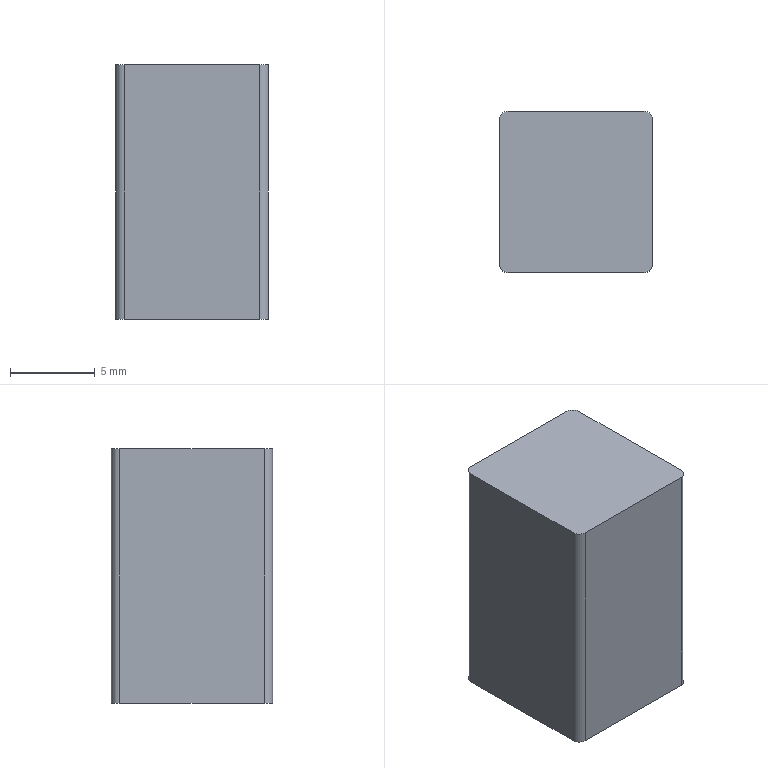Part | NX | features BREP 1 | 1 solid | 10 faces | box 9.003 x 9.506 x 15 mm | volume 1281 mm3 | plane 6 | cylinder 4 | commonest cylinder face diameters 1 x4
STEP:
#1=CARTESIAN_POINT('',(-4.002,4.753,-25.6));
#2=VERTEX_POINT('',#1);
#3=CARTESIAN_POINT('',(-4.502,4.253,-25.6));
#4=VERTEX_POINT('',#3);
#5=CARTESIAN_POINT('',(-4.002,4.253,-25.6));
#6=DIRECTION('',(0.,0.,1.));
#7=DIRECTION('',(1.,0.,0.));
#8=AXIS2_PLACEMENT_3D('',#5,#6,#7);
#9=CIRCLE('',#8,0.5);
#10=EDGE_CURVE('',#2,#4,#9,.T.);
#11=ORIENTED_EDGE('',*,*,#10,.F.);
#12=CARTESIAN_POINT('',(-4.002,4.753,-40.6));
#13=VERTEX_POINT('',#12);
#14=CARTESIAN_POINT('',(-4.002,4.753,-40.6));
#15=DIRECTION('',(0.,0.,1.));
#16=VECTOR('',#15,1000.);
#17=LINE('',#14,#16);
#18=EDGE_CURVE('',#13,#2,#17,.T.);
#19=ORIENTED_EDGE('',*,*,#18,.F.);
#20=CARTESIAN_POINT('',(-4.502,4.253,-40.6));
#21=VERTEX_POINT('',#20);
#22=CARTESIAN_POINT('',(-4.002,4.253,-40.6));
#23=DIRECTION('',(0.,0.,1.));
#24=DIRECTION('',(1.,0.,0.));
#25=AXIS2_PLACEMENT_3D('',#22,#23,#24);
#26=CIRCLE('',#25,0.5);
#27=EDGE_CURVE('',#13,#21,#26,.T.);
#28=ORIENTED_EDGE('',*,*,#27,.T.);
#29=CARTESIAN_POINT('',(-4.502,4.253,-40.6));
#30=DIRECTION('',(0.,0.,1.));
#31=VECTOR('',#30,1000.);
#32=LINE('',#29,#31);
#33=EDGE_CURVE('',#21,#4,#32,.T.);
#34=ORIENTED_EDGE('',*,*,#33,.T.);
#35=EDGE_LOOP('',(#11,#19,#28,#34));
#36=FACE_BOUND('',#35,.T.);
#37=CARTESIAN_POINT('',(-4.002,4.253,-40.6));
#38=DIRECTION('',(0.,0.,1.));
#39=DIRECTION('',(-1.,0.,0.));
#40=AXIS2_PLACEMENT_3D('',#37,#38,#39);
#41=CYLINDRICAL_SURFACE('',#40,0.5);
#42=ADVANCED_FACE('',(#36),#41,.T.);
#43=CARTESIAN_POINT('',(-4.502,-4.253,-25.6));
#44=VERTEX_POINT('',#43);
#45=CARTESIAN_POINT('',(-4.502,-4.253,-25.6));
#46=DIRECTION('',(0.,1.,0.));
#47=VECTOR('',#46,1000.);
#48=LINE('',#45,#47);
#49=EDGE_CURVE('',#44,#4,#48,.T.);
#50=ORIENTED_EDGE('',*,*,#49,.T.);
#51=ORIENTED_EDGE('',*,*,#33,.F.);
#52=CARTESIAN_POINT('',(-4.502,-4.253,-40.6));
#53=VERTEX_POINT('',#52);
#54=CARTESIAN_POINT('',(-4.502,-4.253,-40.6));
#55=DIRECTION('',(0.,1.,0.));
#56=VECTOR('',#55,1000.);
#57=LINE('',#54,#56);
#58=EDGE_CURVE('',#53,#21,#57,.T.);
#59=ORIENTED_EDGE('',*,*,#58,.F.);
#60=CARTESIAN_POINT('',(-4.502,-4.253,-40.6));
#61=DIRECTION('',(0.,0.,1.));
#62=VECTOR('',#61,1000.);
#63=LINE('',#60,#62);
#64=EDGE_CURVE('',#53,#44,#63,.T.);
#65=ORIENTED_EDGE('',*,*,#64,.T.);
#66=EDGE_LOOP('',(#50,#51,#59,#65));
#67=FACE_BOUND('',#66,.T.);
#68=CARTESIAN_POINT('',(-4.502,-4.253,-40.6));
#69=DIRECTION('',(1.,0.,0.));
#70=DIRECTION('',(0.,-1.,0.));
#71=AXIS2_PLACEMENT_3D('',#68,#69,#70);
#72=PLANE('',#71);
#73=ADVANCED_FACE('',(#67),#72,.F.);
#74=CARTESIAN_POINT('',(-4.002,-4.753,-25.6));
#75=VERTEX_POINT('',#74);
#76=CARTESIAN_POINT('',(-4.002,-4.253,-25.6));
#77=DIRECTION('',(0.,0.,1.));
#78=DIRECTION('',(1.,0.,0.));
#79=AXIS2_PLACEMENT_3D('',#76,#77,#78);
#80=CIRCLE('',#79,0.5);
#81=EDGE_CURVE('',#44,#75,#80,.T.);
#82=ORIENTED_EDGE('',*,*,#81,.F.);
#83=ORIENTED_EDGE('',*,*,#64,.F.);
#84=CARTESIAN_POINT('',(-4.002,-4.753,-40.6));
#85=VERTEX_POINT('',#84);
#86=CARTESIAN_POINT('',(-4.002,-4.253,-40.6));
#87=DIRECTION('',(0.,0.,1.));
#88=DIRECTION('',(1.,0.,0.));
#89=AXIS2_PLACEMENT_3D('',#86,#87,#88);
#90=CIRCLE('',#89,0.5);
#91=EDGE_CURVE('',#53,#85,#90,.T.);
#92=ORIENTED_EDGE('',*,*,#91,.T.);
#93=CARTESIAN_POINT('',(-4.002,-4.753,-40.6));
#94=DIRECTION('',(0.,0.,1.));
#95=VECTOR('',#94,1000.);
#96=LINE('',#93,#95);
#97=EDGE_CURVE('',#85,#75,#96,.T.);
#98=ORIENTED_EDGE('',*,*,#97,.T.);
#99=EDGE_LOOP('',(#82,#83,#92,#98));
#100=FACE_BOUND('',#99,.T.);
#101=CARTESIAN_POINT('',(-4.002,-4.253,-40.6));
#102=DIRECTION('',(0.,0.,1.));
#103=DIRECTION('',(-1.,0.,0.));
#104=AXIS2_PLACEMENT_3D('',#101,#102,#103);
#105=CYLINDRICAL_SURFACE('',#104,0.5);
#106=ADVANCED_FACE('',(#100),#105,.T.);
#107=CARTESIAN_POINT('',(4.002,-4.753,-25.6));
#108=VERTEX_POINT('',#107);
#109=CARTESIAN_POINT('',(4.002,-4.753,-25.6));
#110=DIRECTION('',(-1.,0.,0.));
#111=VECTOR('',#110,1000.);
#112=LINE('',#109,#111);
#113=EDGE_CURVE('',#108,#75,#112,.T.);
#114=ORIENTED_EDGE('',*,*,#113,.T.);
#115=ORIENTED_EDGE('',*,*,#97,.F.);
#116=CARTESIAN_POINT('',(4.002,-4.753,-40.6));
#117=VERTEX_POINT('',#116);
#118=CARTESIAN_POINT('',(4.002,-4.753,-40.6));
#119=DIRECTION('',(-1.,0.,0.));
#120=VECTOR('',#119,1000.);
#121=LINE('',#118,#120);
#122=EDGE_CURVE('',#117,#85,#121,.T.);
#123=ORIENTED_EDGE('',*,*,#122,.F.);
#124=CARTESIAN_POINT('',(4.002,-4.753,-40.6));
#125=DIRECTION('',(0.,0.,1.));
#126=VECTOR('',#125,1000.);
#127=LINE('',#124,#126);
#128=EDGE_CURVE('',#117,#108,#127,.T.);
#129=ORIENTED_EDGE('',*,*,#128,.T.);
#130=EDGE_LOOP('',(#114,#115,#123,#129));
#131=FACE_BOUND('',#130,.T.);
#132=CARTESIAN_POINT('',(4.002,-4.753,-40.6));
#133=DIRECTION('',(0.,1.,0.));
#134=DIRECTION('',(1.,0.,0.));
#135=AXIS2_PLACEMENT_3D('',#132,#133,#134);
#136=PLANE('',#135);
#137=ADVANCED_FACE('',(#131),#136,.F.);
#138=CARTESIAN_POINT('',(4.502,-4.253,-25.6));
#139=VERTEX_POINT('',#138);
#140=CARTESIAN_POINT('',(4.002,-4.253,-25.6));
#141=DIRECTION('',(0.,0.,1.));
#142=DIRECTION('',(1.,0.,0.));
#143=AXIS2_PLACEMENT_3D('',#140,#141,#142);
#144=CIRCLE('',#143,0.5);
#145=EDGE_CURVE('',#108,#139,#144,.T.);
#146=ORIENTED_EDGE('',*,*,#145,.F.);
#147=ORIENTED_EDGE('',*,*,#128,.F.);
#148=CARTESIAN_POINT('',(4.502,-4.253,-40.6));
#149=VERTEX_POINT('',#148);
#150=CARTESIAN_POINT('',(4.002,-4.253,-40.6));
#151=DIRECTION('',(0.,0.,1.));
#152=DIRECTION('',(1.,0.,0.));
#153=AXIS2_PLACEMENT_3D('',#150,#151,#152);
#154=CIRCLE('',#153,0.5);
#155=EDGE_CURVE('',#117,#149,#154,.T.);
#156=ORIENTED_EDGE('',*,*,#155,.T.);
#157=CARTESIAN_POINT('',(4.502,-4.253,-40.6));
#158=DIRECTION('',(0.,0.,1.));
#159=VECTOR('',#158,1000.);
#160=LINE('',#157,#159);
#161=EDGE_CURVE('',#149,#139,#160,.T.);
#162=ORIENTED_EDGE('',*,*,#161,.T.);
#163=EDGE_LOOP('',(#146,#147,#156,#162));
#164=FACE_BOUND('',#163,.T.);
#165=CARTESIAN_POINT('',(4.002,-4.253,-40.6));
#166=DIRECTION('',(0.,0.,1.));
#167=DIRECTION('',(-1.,0.,0.));
#168=AXIS2_PLACEMENT_3D('',#165,#166,#167);
#169=CYLINDRICAL_SURFACE('',#168,0.5);
#170=ADVANCED_FACE('',(#164),#169,.T.);
#171=CARTESIAN_POINT('',(4.502,4.253,-25.6));
#172=VERTEX_POINT('',#171);
#173=CARTESIAN_POINT('',(4.502,4.253,-25.6));
#174=DIRECTION('',(0.,-1.,0.));
#175=VECTOR('',#174,1000.);
#176=LINE('',#173,#175);
#177=EDGE_CURVE('',#172,#139,#176,.T.);
#178=ORIENTED_EDGE('',*,*,#177,.T.);
#179=ORIENTED_EDGE('',*,*,#161,.F.);
#180=CARTESIAN_POINT('',(4.502,4.253,-40.6));
#181=VERTEX_POINT('',#180);
#182=CARTESIAN_POINT('',(4.502,4.253,-40.6));
#183=DIRECTION('',(0.,-1.,0.));
#184=VECTOR('',#183,1000.);
#185=LINE('',#182,#184);
#186=EDGE_CURVE('',#181,#149,#185,.T.);
#187=ORIENTED_EDGE('',*,*,#186,.F.);
#188=CARTESIAN_POINT('',(4.502,4.253,-40.6));
#189=DIRECTION('',(0.,0.,1.));
#190=VECTOR('',#189,1000.);
#191=LINE('',#188,#190);
#192=EDGE_CURVE('',#181,#172,#191,.T.);
#193=ORIENTED_EDGE('',*,*,#192,.T.);
#194=EDGE_LOOP('',(#178,#179,#187,#193));
#195=FACE_BOUND('',#194,.T.);
#196=CARTESIAN_POINT('',(4.502,4.253,-40.6));
#197=DIRECTION('',(-1.,0.,0.));
#198=DIRECTION('',(0.,1.,0.));
#199=AXIS2_PLACEMENT_3D('',#196,#197,#198);
#200=PLANE('',#199);
#201=ADVANCED_FACE('',(#195),#200,.F.);
#202=CARTESIAN_POINT('',(4.002,4.753,-25.6));
#203=VERTEX_POINT('',#202);
#204=CARTESIAN_POINT('',(4.002,4.253,-25.6));
#205=DIRECTION('',(0.,0.,1.));
#206=DIRECTION('',(1.,0.,0.));
#207=AXIS2_PLACEMENT_3D('',#204,#205,#206);
#208=CIRCLE('',#207,0.5);
#209=EDGE_CURVE('',#172,#203,#208,.T.);
#210=ORIENTED_EDGE('',*,*,#209,.F.);
#211=ORIENTED_EDGE('',*,*,#192,.F.);
#212=CARTESIAN_POINT('',(4.002,4.753,-40.6));
#213=VERTEX_POINT('',#212);
#214=CARTESIAN_POINT('',(4.002,4.253,-40.6));
#215=DIRECTION('',(0.,0.,1.));
#216=DIRECTION('',(1.,0.,0.));
#217=AXIS2_PLACEMENT_3D('',#214,#215,#216);
#218=CIRCLE('',#217,0.5);
#219=EDGE_CURVE('',#181,#213,#218,.T.);
#220=ORIENTED_EDGE('',*,*,#219,.T.);
#221=CARTESIAN_POINT('',(4.002,4.753,-40.6));
#222=DIRECTION('',(0.,0.,1.));
#223=VECTOR('',#222,1000.);
#224=LINE('',#221,#223);
#225=EDGE_CURVE('',#213,#203,#224,.T.);
#226=ORIENTED_EDGE('',*,*,#225,.T.);
#227=EDGE_LOOP('',(#210,#211,#220,#226));
#228=FACE_BOUND('',#227,.T.);
#229=CARTESIAN_POINT('',(4.002,4.253,-40.6));
#230=DIRECTION('',(0.,0.,1.));
#231=DIRECTION('',(-1.,0.,0.));
#232=AXIS2_PLACEMENT_3D('',#229,#230,#231);
#233=CYLINDRICAL_SURFACE('',#232,0.5);
#234=ADVANCED_FACE('',(#228),#233,.T.);
#235=CARTESIAN_POINT('',(-4.002,4.753,-25.6));
#236=DIRECTION('',(1.,0.,0.));
#237=VECTOR('',#236,1000.);
#238=LINE('',#235,#237);
#239=EDGE_CURVE('',#2,#203,#238,.T.);
#240=ORIENTED_EDGE('',*,*,#239,.T.);
#241=ORIENTED_EDGE('',*,*,#225,.F.);
#242=CARTESIAN_POINT('',(-4.002,4.753,-40.6));
#243=DIRECTION('',(1.,0.,0.));
#244=VECTOR('',#243,1000.);
#245=LINE('',#242,#244);
#246=EDGE_CURVE('',#13,#213,#245,.T.);
#247=ORIENTED_EDGE('',*,*,#246,.F.);
#248=ORIENTED_EDGE('',*,*,#18,.T.);
#249=EDGE_LOOP('',(#240,#241,#247,#248));
#250=FACE_BOUND('',#249,.T.);
#251=CARTESIAN_POINT('',(-4.002,4.753,-40.6));
#252=DIRECTION('',(0.,-1.,0.));
#253=DIRECTION('',(0.,0.,1.));
#254=AXIS2_PLACEMENT_3D('',#251,#252,#253);
#255=PLANE('',#254);
#256=ADVANCED_FACE('',(#250),#255,.F.);
#257=ORIENTED_EDGE('',*,*,#27,.F.);
#258=ORIENTED_EDGE('',*,*,#246,.T.);
#259=ORIENTED_EDGE('',*,*,#219,.F.);
#260=ORIENTED_EDGE('',*,*,#186,.T.);
#261=ORIENTED_EDGE('',*,*,#155,.F.);
#262=ORIENTED_EDGE('',*,*,#122,.T.);
#263=ORIENTED_EDGE('',*,*,#91,.F.);
#264=ORIENTED_EDGE('',*,*,#58,.T.);
#265=EDGE_LOOP('',(#257,#258,#259,#260,#261,#262,#263,#264));
#266=FACE_BOUND('',#265,.T.);
#267=CARTESIAN_POINT('',(-4.002,4.253,-40.6));
#268=DIRECTION('',(0.,0.,1.));
#269=DIRECTION('',(-1.,0.,0.));
#270=AXIS2_PLACEMENT_3D('',#267,#268,#269);
#271=PLANE('',#270);
#272=ADVANCED_FACE('',(#266),#271,.F.);
#273=ORIENTED_EDGE('',*,*,#10,.T.);
#274=ORIENTED_EDGE('',*,*,#49,.F.);
#275=ORIENTED_EDGE('',*,*,#81,.T.);
#276=ORIENTED_EDGE('',*,*,#113,.F.);
#277=ORIENTED_EDGE('',*,*,#145,.T.);
#278=ORIENTED_EDGE('',*,*,#177,.F.);
#279=ORIENTED_EDGE('',*,*,#209,.T.);
#280=ORIENTED_EDGE('',*,*,#239,.F.);
#281=EDGE_LOOP('',(#273,#274,#275,#276,#277,#278,#279,#280));
#282=FACE_BOUND('',#281,.T.);
#283=CARTESIAN_POINT('',(-4.002,4.253,-25.6));
#284=DIRECTION('',(0.,0.,1.));
#285=DIRECTION('',(-1.,0.,0.));
#286=AXIS2_PLACEMENT_3D('',#283,#284,#285);
#287=PLANE('',#286);
#288=ADVANCED_FACE('',(#282),#287,.T.);
#289=CLOSED_SHELL('',(#42,#73,#106,#137,#170,#201,#234,#256,#272,#288));
#290=MANIFOLD_SOLID_BREP('',#289);
#291=(LENGTH_UNIT()NAMED_UNIT(*)SI_UNIT(.MILLI.,.METRE.));
#292=UNCERTAINTY_MEASURE_WITH_UNIT(LENGTH_MEASURE(0.00001),#291,'','');
#293=(NAMED_UNIT(*)PLANE_ANGLE_UNIT()SI_UNIT($,.RADIAN.));
#294=(NAMED_UNIT(*)SI_UNIT($,.STERADIAN.)SOLID_ANGLE_UNIT());
#295=(GEOMETRIC_REPRESENTATION_CONTEXT(3)GLOBAL_UNCERTAINTY_ASSIGNED_CONTEXT((#292))GLOBAL_UNIT_ASSIGNED_CONTEXT((#291,#293,#294))REPRESENTATION_CONTEXT('',''));
#296=ADVANCED_BREP_SHAPE_REPRESENTATION('',(#290),#295);